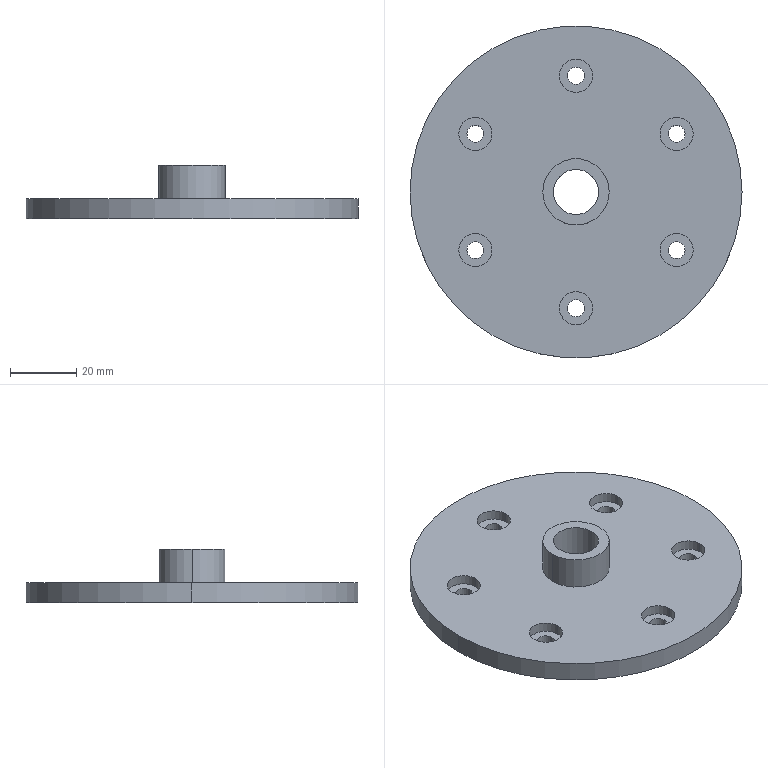Part | NX | 1 solid | 38 faces | box 100 x 100 x 16 mm | volume 46160 mm3 | cylinder 29 | plane 9 | commonest cylinder face diameters 5.1 x12 10 x12 20 x2 100 x2 13.6 x1
STEP:
#1=CARTESIAN_POINT('',(5.,-35.,3.));
#2=VERTEX_POINT('',#1);
#3=CARTESIAN_POINT('',(-5.,-35.,3.));
#4=VERTEX_POINT('',#3);
#5=CARTESIAN_POINT('',(0.,-35.,3.));
#6=DIRECTION('',(0.,0.,1.));
#7=DIRECTION('',(1.,0.,0.));
#8=AXIS2_PLACEMENT_3D('',#5,#6,#7);
#9=CIRCLE('',#8,5.);
#10=EDGE_CURVE('',#2,#4,#9,.T.);
#11=ORIENTED_EDGE('',*,*,#10,.T.);
#12=CARTESIAN_POINT('',(0.,-35.,3.));
#13=DIRECTION('',(0.,0.,1.));
#14=DIRECTION('',(1.,0.,0.));
#15=AXIS2_PLACEMENT_3D('',#12,#13,#14);
#16=CIRCLE('',#15,5.);
#17=EDGE_CURVE('',#4,#2,#16,.T.);
#18=ORIENTED_EDGE('',*,*,#17,.T.);
#19=EDGE_LOOP('',(#11,#18));
#20=FACE_BOUND('',#19,.T.);
#21=CARTESIAN_POINT('',(-2.55,-35.,3.));
#22=VERTEX_POINT('',#21);
#23=CARTESIAN_POINT('',(2.55,-35.,3.));
#24=VERTEX_POINT('',#23);
#25=CARTESIAN_POINT('',(0.,-35.,3.));
#26=DIRECTION('',(0.,0.,1.));
#27=DIRECTION('',(1.,0.,0.));
#28=AXIS2_PLACEMENT_3D('',#25,#26,#27);
#29=CIRCLE('',#28,2.55);
#30=EDGE_CURVE('',#22,#24,#29,.T.);
#31=ORIENTED_EDGE('',*,*,#30,.F.);
#32=CARTESIAN_POINT('',(0.,-35.,3.));
#33=DIRECTION('',(0.,0.,1.));
#34=DIRECTION('',(1.,0.,0.));
#35=AXIS2_PLACEMENT_3D('',#32,#33,#34);
#36=CIRCLE('',#35,2.55);
#37=EDGE_CURVE('',#24,#22,#36,.T.);
#38=ORIENTED_EDGE('',*,*,#37,.F.);
#39=EDGE_LOOP('',(#31,#38));
#40=FACE_BOUND('',#39,.T.);
#41=CARTESIAN_POINT('',(0.,-35.,3.));
#42=DIRECTION('',(0.,0.,1.));
#43=DIRECTION('',(1.,0.,0.));
#44=AXIS2_PLACEMENT_3D('',#41,#42,#43);
#45=PLANE('',#44);
#46=ADVANCED_FACE('',(#20,#40),#45,.T.);
#47=CARTESIAN_POINT('',(-5.,-35.,6.));
#48=VERTEX_POINT('',#47);
#49=CARTESIAN_POINT('',(-5.,-35.,3.));
#50=DIRECTION('',(0.,0.,1.));
#51=VECTOR('',#50,1000.);
#52=LINE('',#49,#51);
#53=EDGE_CURVE('',#4,#48,#52,.T.);
#54=ORIENTED_EDGE('',*,*,#53,.F.);
#55=ORIENTED_EDGE('',*,*,#10,.F.);
#56=CARTESIAN_POINT('',(5.,-35.,6.));
#57=VERTEX_POINT('',#56);
#58=CARTESIAN_POINT('',(5.,-35.,3.));
#59=DIRECTION('',(0.,0.,1.));
#60=VECTOR('',#59,1000.);
#61=LINE('',#58,#60);
#62=EDGE_CURVE('',#2,#57,#61,.T.);
#63=ORIENTED_EDGE('',*,*,#62,.T.);
#64=CARTESIAN_POINT('',(0.,-35.,6.));
#65=DIRECTION('',(0.,0.,1.));
#66=DIRECTION('',(1.,0.,0.));
#67=AXIS2_PLACEMENT_3D('',#64,#65,#66);
#68=CIRCLE('',#67,5.);
#69=EDGE_CURVE('',#57,#48,#68,.T.);
#70=ORIENTED_EDGE('',*,*,#69,.T.);
#71=EDGE_LOOP('',(#54,#55,#63,#70));
#72=FACE_BOUND('',#71,.T.);
#73=CARTESIAN_POINT('',(0.,-35.,3.));
#74=DIRECTION('',(0.,0.,1.));
#75=DIRECTION('',(1.,0.,0.));
#76=AXIS2_PLACEMENT_3D('',#73,#74,#75);
#77=CYLINDRICAL_SURFACE('',#76,5.);
#78=ADVANCED_FACE('',(#72),#77,.F.);
#79=CARTESIAN_POINT('',(5.,35.,3.));
#80=VERTEX_POINT('',#79);
#81=CARTESIAN_POINT('',(-5.,35.,3.));
#82=VERTEX_POINT('',#81);
#83=CARTESIAN_POINT('',(0.,35.,3.));
#84=DIRECTION('',(0.,0.,1.));
#85=DIRECTION('',(1.,0.,0.));
#86=AXIS2_PLACEMENT_3D('',#83,#84,#85);
#87=CIRCLE('',#86,5.);
#88=EDGE_CURVE('',#80,#82,#87,.T.);
#89=ORIENTED_EDGE('',*,*,#88,.T.);
#90=CARTESIAN_POINT('',(0.,35.,3.));
#91=DIRECTION('',(0.,0.,1.));
#92=DIRECTION('',(1.,0.,0.));
#93=AXIS2_PLACEMENT_3D('',#90,#91,#92);
#94=CIRCLE('',#93,5.);
#95=EDGE_CURVE('',#82,#80,#94,.T.);
#96=ORIENTED_EDGE('',*,*,#95,.T.);
#97=EDGE_LOOP('',(#89,#96));
#98=FACE_BOUND('',#97,.T.);
#99=CARTESIAN_POINT('',(-2.55,35.,3.));
#100=VERTEX_POINT('',#99);
#101=CARTESIAN_POINT('',(2.55,35.,3.));
#102=VERTEX_POINT('',#101);
#103=CARTESIAN_POINT('',(0.,35.,3.));
#104=DIRECTION('',(0.,0.,1.));
#105=DIRECTION('',(1.,0.,0.));
#106=AXIS2_PLACEMENT_3D('',#103,#104,#105);
#107=CIRCLE('',#106,2.55);
#108=EDGE_CURVE('',#100,#102,#107,.T.);
#109=ORIENTED_EDGE('',*,*,#108,.F.);
#110=CARTESIAN_POINT('',(0.,35.,3.));
#111=DIRECTION('',(0.,0.,1.));
#112=DIRECTION('',(1.,0.,0.));
#113=AXIS2_PLACEMENT_3D('',#110,#111,#112);
#114=CIRCLE('',#113,2.55);
#115=EDGE_CURVE('',#102,#100,#114,.T.);
#116=ORIENTED_EDGE('',*,*,#115,.F.);
#117=EDGE_LOOP('',(#109,#116));
#118=FACE_BOUND('',#117,.T.);
#119=CARTESIAN_POINT('',(0.,35.,3.));
#120=DIRECTION('',(0.,0.,1.));
#121=DIRECTION('',(1.,0.,0.));
#122=AXIS2_PLACEMENT_3D('',#119,#120,#121);
#123=PLANE('',#122);
#124=ADVANCED_FACE('',(#98,#118),#123,.T.);
#125=CARTESIAN_POINT('',(-5.,35.,6.));
#126=VERTEX_POINT('',#125);
#127=CARTESIAN_POINT('',(-5.,35.,3.));
#128=DIRECTION('',(0.,0.,1.));
#129=VECTOR('',#128,1000.);
#130=LINE('',#127,#129);
#131=EDGE_CURVE('',#82,#126,#130,.T.);
#132=ORIENTED_EDGE('',*,*,#131,.F.);
#133=ORIENTED_EDGE('',*,*,#88,.F.);
#134=CARTESIAN_POINT('',(5.,35.,6.));
#135=VERTEX_POINT('',#134);
#136=CARTESIAN_POINT('',(5.,35.,3.));
#137=DIRECTION('',(0.,0.,1.));
#138=VECTOR('',#137,1000.);
#139=LINE('',#136,#138);
#140=EDGE_CURVE('',#80,#135,#139,.T.);
#141=ORIENTED_EDGE('',*,*,#140,.T.);
#142=CARTESIAN_POINT('',(0.,35.,6.));
#143=DIRECTION('',(0.,0.,1.));
#144=DIRECTION('',(1.,0.,0.));
#145=AXIS2_PLACEMENT_3D('',#142,#143,#144);
#146=CIRCLE('',#145,5.);
#147=EDGE_CURVE('',#135,#126,#146,.T.);
#148=ORIENTED_EDGE('',*,*,#147,.T.);
#149=EDGE_LOOP('',(#132,#133,#141,#148));
#150=FACE_BOUND('',#149,.T.);
#151=CARTESIAN_POINT('',(0.,35.,3.));
#152=DIRECTION('',(0.,0.,1.));
#153=DIRECTION('',(1.,0.,0.));
#154=AXIS2_PLACEMENT_3D('',#151,#152,#153);
#155=CYLINDRICAL_SURFACE('',#154,5.);
#156=ADVANCED_FACE('',(#150),#155,.F.);
#157=CARTESIAN_POINT('',(35.311,17.5,3.));
#158=VERTEX_POINT('',#157);
#159=CARTESIAN_POINT('',(25.311,17.5,3.));
#160=VERTEX_POINT('',#159);
#161=CARTESIAN_POINT('',(30.311,17.5,3.));
#162=DIRECTION('',(0.,0.,1.));
#163=DIRECTION('',(1.,0.,0.));
#164=AXIS2_PLACEMENT_3D('',#161,#162,#163);
#165=CIRCLE('',#164,5.);
#166=EDGE_CURVE('',#158,#160,#165,.T.);
#167=ORIENTED_EDGE('',*,*,#166,.T.);
#168=CARTESIAN_POINT('',(30.311,17.5,3.));
#169=DIRECTION('',(0.,0.,1.));
#170=DIRECTION('',(1.,0.,0.));
#171=AXIS2_PLACEMENT_3D('',#168,#169,#170);
#172=CIRCLE('',#171,5.);
#173=EDGE_CURVE('',#160,#158,#172,.T.);
#174=ORIENTED_EDGE('',*,*,#173,.T.);
#175=EDGE_LOOP('',(#167,#174));
#176=FACE_BOUND('',#175,.T.);
#177=CARTESIAN_POINT('',(27.761,17.5,3.));
#178=VERTEX_POINT('',#177);
#179=CARTESIAN_POINT('',(32.861,17.5,3.));
#180=VERTEX_POINT('',#179);
#181=CARTESIAN_POINT('',(30.311,17.5,3.));
#182=DIRECTION('',(0.,0.,1.));
#183=DIRECTION('',(1.,0.,0.));
#184=AXIS2_PLACEMENT_3D('',#181,#182,#183);
#185=CIRCLE('',#184,2.55);
#186=EDGE_CURVE('',#178,#180,#185,.T.);
#187=ORIENTED_EDGE('',*,*,#186,.F.);
#188=CARTESIAN_POINT('',(30.311,17.5,3.));
#189=DIRECTION('',(0.,0.,1.));
#190=DIRECTION('',(1.,0.,0.));
#191=AXIS2_PLACEMENT_3D('',#188,#189,#190);
#192=CIRCLE('',#191,2.55);
#193=EDGE_CURVE('',#180,#178,#192,.T.);
#194=ORIENTED_EDGE('',*,*,#193,.F.);
#195=EDGE_LOOP('',(#187,#194));
#196=FACE_BOUND('',#195,.T.);
#197=CARTESIAN_POINT('',(30.311,17.5,3.));
#198=DIRECTION('',(0.,0.,1.));
#199=DIRECTION('',(1.,0.,0.));
#200=AXIS2_PLACEMENT_3D('',#197,#198,#199);
#201=PLANE('',#200);
#202=ADVANCED_FACE('',(#176,#196),#201,.T.);
#203=CARTESIAN_POINT('',(25.311,17.5,6.));
#204=VERTEX_POINT('',#203);
#205=CARTESIAN_POINT('',(25.311,17.5,3.));
#206=DIRECTION('',(0.,0.,1.));
#207=VECTOR('',#206,1000.);
#208=LINE('',#205,#207);
#209=EDGE_CURVE('',#160,#204,#208,.T.);
#210=ORIENTED_EDGE('',*,*,#209,.F.);
#211=ORIENTED_EDGE('',*,*,#166,.F.);
#212=CARTESIAN_POINT('',(35.311,17.5,6.));
#213=VERTEX_POINT('',#212);
#214=CARTESIAN_POINT('',(35.311,17.5,3.));
#215=DIRECTION('',(0.,0.,1.));
#216=VECTOR('',#215,1000.);
#217=LINE('',#214,#216);
#218=EDGE_CURVE('',#158,#213,#217,.T.);
#219=ORIENTED_EDGE('',*,*,#218,.T.);
#220=CARTESIAN_POINT('',(30.311,17.5,6.));
#221=DIRECTION('',(0.,0.,1.));
#222=DIRECTION('',(1.,0.,0.));
#223=AXIS2_PLACEMENT_3D('',#220,#221,#222);
#224=CIRCLE('',#223,5.);
#225=EDGE_CURVE('',#213,#204,#224,.T.);
#226=ORIENTED_EDGE('',*,*,#225,.T.);
#227=EDGE_LOOP('',(#210,#211,#219,#226));
#228=FACE_BOUND('',#227,.T.);
#229=CARTESIAN_POINT('',(30.311,17.5,3.));
#230=DIRECTION('',(0.,0.,1.));
#231=DIRECTION('',(1.,0.,0.));
#232=AXIS2_PLACEMENT_3D('',#229,#230,#231);
#233=CYLINDRICAL_SURFACE('',#232,5.);
#234=ADVANCED_FACE('',(#228),#233,.F.);
#235=CARTESIAN_POINT('',(35.311,-17.5,3.));
#236=VERTEX_POINT('',#235);
#237=CARTESIAN_POINT('',(25.311,-17.5,3.));
#238=VERTEX_POINT('',#237);
#239=CARTESIAN_POINT('',(30.311,-17.5,3.));
#240=DIRECTION('',(0.,0.,1.));
#241=DIRECTION('',(1.,0.,0.));
#242=AXIS2_PLACEMENT_3D('',#239,#240,#241);
#243=CIRCLE('',#242,5.);
#244=EDGE_CURVE('',#236,#238,#243,.T.);
#245=ORIENTED_EDGE('',*,*,#244,.T.);
#246=CARTESIAN_POINT('',(30.311,-17.5,3.));
#247=DIRECTION('',(0.,0.,1.));
#248=DIRECTION('',(1.,0.,0.));
#249=AXIS2_PLACEMENT_3D('',#246,#247,#248);
#250=CIRCLE('',#249,5.);
#251=EDGE_CURVE('',#238,#236,#250,.T.);
#252=ORIENTED_EDGE('',*,*,#251,.T.);
#253=EDGE_LOOP('',(#245,#252));
#254=FACE_BOUND('',#253,.T.);
#255=CARTESIAN_POINT('',(27.761,-17.5,3.));
#256=VERTEX_POINT('',#255);
#257=CARTESIAN_POINT('',(32.861,-17.5,3.));
#258=VERTEX_POINT('',#257);
#259=CARTESIAN_POINT('',(30.311,-17.5,3.));
#260=DIRECTION('',(0.,0.,1.));
#261=DIRECTION('',(1.,0.,0.));
#262=AXIS2_PLACEMENT_3D('',#259,#260,#261);
#263=CIRCLE('',#262,2.55);
#264=EDGE_CURVE('',#256,#258,#263,.T.);
#265=ORIENTED_EDGE('',*,*,#264,.F.);
#266=CARTESIAN_POINT('',(30.311,-17.5,3.));
#267=DIRECTION('',(0.,0.,1.));
#268=DIRECTION('',(1.,0.,0.));
#269=AXIS2_PLACEMENT_3D('',#266,#267,#268);
#270=CIRCLE('',#269,2.55);
#271=EDGE_CURVE('',#258,#256,#270,.T.);
#272=ORIENTED_EDGE('',*,*,#271,.F.);
#273=EDGE_LOOP('',(#265,#272));
#274=FACE_BOUND('',#273,.T.);
#275=CARTESIAN_POINT('',(30.311,-17.5,3.));
#276=DIRECTION('',(0.,0.,1.));
#277=DIRECTION('',(1.,0.,0.));
#278=AXIS2_PLACEMENT_3D('',#275,#276,#277);
#279=PLANE('',#278);
#280=ADVANCED_FACE('',(#254,#274),#279,.T.);
#281=CARTESIAN_POINT('',(25.311,-17.5,6.));
#282=VERTEX_POINT('',#281);
#283=CARTESIAN_POINT('',(25.311,-17.5,3.));
#284=DIRECTION('',(0.,0.,1.));
#285=VECTOR('',#284,1000.);
#286=LINE('',#283,#285);
#287=EDGE_CURVE('',#238,#282,#286,.T.);
#288=ORIENTED_EDGE('',*,*,#287,.F.);
#289=ORIENTED_EDGE('',*,*,#244,.F.);
#290=CARTESIAN_POINT('',(35.311,-17.5,6.));
#291=VERTEX_POINT('',#290);
#292=CARTESIAN_POINT('',(35.311,-17.5,3.));
#293=DIRECTION('',(0.,0.,1.));
#294=VECTOR('',#293,1000.);
#295=LINE('',#292,#294);
#296=EDGE_CURVE('',#236,#291,#295,.T.);
#297=ORIENTED_EDGE('',*,*,#296,.T.);
#298=CARTESIAN_POINT('',(30.311,-17.5,6.));
#299=DIRECTION('',(0.,0.,1.));
#300=DIRECTION('',(1.,0.,0.));
#301=AXIS2_PLACEMENT_3D('',#298,#299,#300);
#302=CIRCLE('',#301,5.);
#303=EDGE_CURVE('',#291,#282,#302,.T.);
#304=ORIENTED_EDGE('',*,*,#303,.T.);
#305=EDGE_LOOP('',(#288,#289,#297,#304));
#306=FACE_BOUND('',#305,.T.);
#307=CARTESIAN_POINT('',(30.311,-17.5,3.));
#308=DIRECTION('',(0.,0.,1.));
#309=DIRECTION('',(1.,0.,0.));
#310=AXIS2_PLACEMENT_3D('',#307,#308,#309);
#311=CYLINDRICAL_SURFACE('',#310,5.);
#312=ADVANCED_FACE('',(#306),#311,.F.);
#313=CARTESIAN_POINT('',(-25.311,-17.5,3.));
#314=VERTEX_POINT('',#313);
#315=CARTESIAN_POINT('',(-35.311,-17.5,3.));
#316=VERTEX_POINT('',#315);
#317=CARTESIAN_POINT('',(-30.311,-17.5,3.));
#318=DIRECTION('',(0.,0.,1.));
#319=DIRECTION('',(1.,0.,0.));
#320=AXIS2_PLACEMENT_3D('',#317,#318,#319);
#321=CIRCLE('',#320,5.);
#322=EDGE_CURVE('',#314,#316,#321,.T.);
#323=ORIENTED_EDGE('',*,*,#322,.T.);
#324=CARTESIAN_POINT('',(-30.311,-17.5,3.));
#325=DIRECTION('',(0.,0.,1.));
#326=DIRECTION('',(1.,0.,0.));
#327=AXIS2_PLACEMENT_3D('',#324,#325,#326);
#328=CIRCLE('',#327,5.);
#329=EDGE_CURVE('',#316,#314,#328,.T.);
#330=ORIENTED_EDGE('',*,*,#329,.T.);
#331=EDGE_LOOP('',(#323,#330));
#332=FACE_BOUND('',#331,.T.);
#333=CARTESIAN_POINT('',(-32.861,-17.5,3.));
#334=VERTEX_POINT('',#333);
#335=CARTESIAN_POINT('',(-27.761,-17.5,3.));
#336=VERTEX_POINT('',#335);
#337=CARTESIAN_POINT('',(-30.311,-17.5,3.));
#338=DIRECTION('',(0.,0.,1.));
#339=DIRECTION('',(1.,0.,0.));
#340=AXIS2_PLACEMENT_3D('',#337,#338,#339);
#341=CIRCLE('',#340,2.55);
#342=EDGE_CURVE('',#334,#336,#341,.T.);
#343=ORIENTED_EDGE('',*,*,#342,.F.);
#344=CARTESIAN_POINT('',(-30.311,-17.5,3.));
#345=DIRECTION('',(0.,0.,1.));
#346=DIRECTION('',(1.,0.,0.));
#347=AXIS2_PLACEMENT_3D('',#344,#345,#346);
#348=CIRCLE('',#347,2.55);
#349=EDGE_CURVE('',#336,#334,#348,.T.);
#350=ORIENTED_EDGE('',*,*,#349,.F.);
#351=EDGE_LOOP('',(#343,#350));
#352=FACE_BOUND('',#351,.T.);
#353=CARTESIAN_POINT('',(-30.311,-17.5,3.));
#354=DIRECTION('',(0.,0.,1.));
#355=DIRECTION('',(1.,0.,0.));
#356=AXIS2_PLACEMENT_3D('',#353,#354,#355);
#357=PLANE('',#356);
#358=ADVANCED_FACE('',(#332,#352),#357,.T.);
#359=CARTESIAN_POINT('',(-35.311,-17.5,6.));
#360=VERTEX_POINT('',#359);
#361=CARTESIAN_POINT('',(-35.311,-17.5,3.));
#362=DIRECTION('',(0.,0.,1.));
#363=VECTOR('',#362,1000.);
#364=LINE('',#361,#363);
#365=EDGE_CURVE('',#316,#360,#364,.T.);
#366=ORIENTED_EDGE('',*,*,#365,.F.);
#367=ORIENTED_EDGE('',*,*,#322,.F.);
#368=CARTESIAN_POINT('',(-25.311,-17.5,6.));
#369=VERTEX_POINT('',#368);
#370=CARTESIAN_POINT('',(-25.311,-17.5,3.));
#371=DIRECTION('',(0.,0.,1.));
#372=VECTOR('',#371,1000.);
#373=LINE('',#370,#372);
#374=EDGE_CURVE('',#314,#369,#373,.T.);
#375=ORIENTED_EDGE('',*,*,#374,.T.);
#376=CARTESIAN_POINT('',(-30.311,-17.5,6.));
#377=DIRECTION('',(0.,0.,1.));
#378=DIRECTION('',(1.,0.,0.));
#379=AXIS2_PLACEMENT_3D('',#376,#377,#378);
#380=CIRCLE('',#379,5.);
#381=EDGE_CURVE('',#369,#360,#380,.T.);
#382=ORIENTED_EDGE('',*,*,#381,.T.);
#383=EDGE_LOOP('',(#366,#367,#375,#382));
#384=FACE_BOUND('',#383,.T.);
#385=CARTESIAN_POINT('',(-30.311,-17.5,3.));
#386=DIRECTION('',(0.,0.,1.));
#387=DIRECTION('',(1.,0.,0.));
#388=AXIS2_PLACEMENT_3D('',#385,#386,#387);
#389=CYLINDRICAL_SURFACE('',#388,5.);
#390=ADVANCED_FACE('',(#384),#389,.F.);
#391=CARTESIAN_POINT('',(-25.311,17.5,3.));
#392=VERTEX_POINT('',#391);
#393=CARTESIAN_POINT('',(-35.311,17.5,3.));
#394=VERTEX_POINT('',#393);
#395=CARTESIAN_POINT('',(-30.311,17.5,3.));
#396=DIRECTION('',(0.,0.,1.));
#397=DIRECTION('',(1.,0.,0.));
#398=AXIS2_PLACEMENT_3D('',#395,#396,#397);
#399=CIRCLE('',#398,5.);
#400=EDGE_CURVE('',#392,#394,#399,.T.);
#401=ORIENTED_EDGE('',*,*,#400,.T.);
#402=CARTESIAN_POINT('',(-30.311,17.5,3.));
#403=DIRECTION('',(0.,0.,1.));
#404=DIRECTION('',(1.,0.,0.));
#405=AXIS2_PLACEMENT_3D('',#402,#403,#404);
#406=CIRCLE('',#405,5.);
#407=EDGE_CURVE('',#394,#392,#406,.T.);
#408=ORIENTED_EDGE('',*,*,#407,.T.);
#409=EDGE_LOOP('',(#401,#408));
#410=FACE_BOUND('',#409,.T.);
#411=CARTESIAN_POINT('',(-32.861,17.5,3.));
#412=VERTEX_POINT('',#411);
#413=CARTESIAN_POINT('',(-27.761,17.5,3.));
#414=VERTEX_POINT('',#413);
#415=CARTESIAN_POINT('',(-30.311,17.5,3.));
#416=DIRECTION('',(0.,0.,1.));
#417=DIRECTION('',(1.,0.,0.));
#418=AXIS2_PLACEMENT_3D('',#415,#416,#417);
#419=CIRCLE('',#418,2.55);
#420=EDGE_CURVE('',#412,#414,#419,.T.);
#421=ORIENTED_EDGE('',*,*,#420,.F.);
#422=CARTESIAN_POINT('',(-30.311,17.5,3.));
#423=DIRECTION('',(0.,0.,1.));
#424=DIRECTION('',(1.,0.,0.));
#425=AXIS2_PLACEMENT_3D('',#422,#423,#424);
#426=CIRCLE('',#425,2.55);
#427=EDGE_CURVE('',#414,#412,#426,.T.);
#428=ORIENTED_EDGE('',*,*,#427,.F.);
#429=EDGE_LOOP('',(#421,#428));
#430=FACE_BOUND('',#429,.T.);
#431=CARTESIAN_POINT('',(-30.311,17.5,3.));
#432=DIRECTION('',(0.,0.,1.));
#433=DIRECTION('',(1.,0.,0.));
#434=AXIS2_PLACEMENT_3D('',#431,#432,#433);
#435=PLANE('',#434);
#436=ADVANCED_FACE('',(#410,#430),#435,.T.);
#437=CARTESIAN_POINT('',(-35.311,17.5,6.));
#438=VERTEX_POINT('',#437);
#439=CARTESIAN_POINT('',(-35.311,17.5,3.));
#440=DIRECTION('',(0.,0.,1.));
#441=VECTOR('',#440,1000.);
#442=LINE('',#439,#441);
#443=EDGE_CURVE('',#394,#438,#442,.T.);
#444=ORIENTED_EDGE('',*,*,#443,.F.);
#445=ORIENTED_EDGE('',*,*,#400,.F.);
#446=CARTESIAN_POINT('',(-25.311,17.5,6.));
#447=VERTEX_POINT('',#446);
#448=CARTESIAN_POINT('',(-25.311,17.5,3.));
#449=DIRECTION('',(0.,0.,1.));
#450=VECTOR('',#449,1000.);
#451=LINE('',#448,#450);
#452=EDGE_CURVE('',#392,#447,#451,.T.);
#453=ORIENTED_EDGE('',*,*,#452,.T.);
#454=CARTESIAN_POINT('',(-30.311,17.5,6.));
#455=DIRECTION('',(0.,0.,1.));
#456=DIRECTION('',(1.,0.,0.));
#457=AXIS2_PLACEMENT_3D('',#454,#455,#456);
#458=CIRCLE('',#457,5.);
#459=EDGE_CURVE('',#447,#438,#458,.T.);
#460=ORIENTED_EDGE('',*,*,#459,.T.);
#461=EDGE_LOOP('',(#444,#445,#453,#460));
#462=FACE_BOUND('',#461,.T.);
#463=CARTESIAN_POINT('',(-30.311,17.5,3.));
#464=DIRECTION('',(0.,0.,1.));
#465=DIRECTION('',(1.,0.,0.));
#466=AXIS2_PLACEMENT_3D('',#463,#464,#465);
#467=CYLINDRICAL_SURFACE('',#466,5.);
#468=ADVANCED_FACE('',(#462),#467,.F.);
#469=CARTESIAN_POINT('',(10.,0.,16.));
#470=VERTEX_POINT('',#469);
#471=CARTESIAN_POINT('',(10.,0.,6.));
#472=VERTEX_POINT('',#471);
#473=CARTESIAN_POINT('',(10.,0.,16.));
#474=DIRECTION('',(0.,0.,-1.));
#475=VECTOR('',#474,1000.);
#476=LINE('',#473,#475);
#477=EDGE_CURVE('',#470,#472,#476,.T.);
#478=ORIENTED_EDGE('',*,*,#477,.F.);
#479=CARTESIAN_POINT('',(-10.,0.,16.));
#480=VERTEX_POINT('',#479);
#481=CARTESIAN_POINT('',(0.,0.,16.));
#482=DIRECTION('',(0.,0.,1.));
#483=DIRECTION('',(1.,0.,0.));
#484=AXIS2_PLACEMENT_3D('',#481,#482,#483);
#485=CIRCLE('',#484,10.);
#486=EDGE_CURVE('',#480,#470,#485,.T.);
#487=ORIENTED_EDGE('',*,*,#486,.F.);
#488=CARTESIAN_POINT('',(-10.,0.,6.));
#489=VERTEX_POINT('',#488);
#490=CARTESIAN_POINT('',(-10.,0.,16.));
#491=DIRECTION('',(0.,0.,-1.));
#492=VECTOR('',#491,1000.);
#493=LINE('',#490,#492);
#494=EDGE_CURVE('',#480,#489,#493,.T.);
#495=ORIENTED_EDGE('',*,*,#494,.T.);
#496=CARTESIAN_POINT('',(0.,0.,6.));
#497=DIRECTION('',(0.,0.,1.));
#498=DIRECTION('',(1.,0.,0.));
#499=AXIS2_PLACEMENT_3D('',#496,#497,#498);
#500=CIRCLE('',#499,10.);
#501=EDGE_CURVE('',#489,#472,#500,.T.);
#502=ORIENTED_EDGE('',*,*,#501,.T.);
#503=EDGE_LOOP('',(#478,#487,#495,#502));
#504=FACE_BOUND('',#503,.T.);
#505=CARTESIAN_POINT('',(0.,0.,16.));
#506=DIRECTION('',(0.,0.,-1.));
#507=DIRECTION('',(-1.,0.,0.));
#508=AXIS2_PLACEMENT_3D('',#505,#506,#507);
#509=CYLINDRICAL_SURFACE('',#508,10.);
#510=ADVANCED_FACE('',(#504),#509,.T.);
#511=CARTESIAN_POINT('',(6.8,0.,16.));
#512=VERTEX_POINT('',#511);
#513=CARTESIAN_POINT('',(0.,0.,16.));
#514=DIRECTION('',(0.,0.,1.));
#515=DIRECTION('',(1.,0.,0.));
#516=AXIS2_PLACEMENT_3D('',#513,#514,#515);
#517=CIRCLE('',#516,6.8);
#518=EDGE_CURVE('',#512,#512,#517,.T.);
#519=ORIENTED_EDGE('',*,*,#518,.F.);
#520=EDGE_LOOP('',(#519));
#521=FACE_BOUND('',#520,.T.);
#522=ORIENTED_EDGE('',*,*,#486,.T.);
#523=CARTESIAN_POINT('',(0.,0.,16.));
#524=DIRECTION('',(0.,0.,1.));
#525=DIRECTION('',(1.,0.,0.));
#526=AXIS2_PLACEMENT_3D('',#523,#524,#525);
#527=CIRCLE('',#526,10.);
#528=EDGE_CURVE('',#470,#480,#527,.T.);
#529=ORIENTED_EDGE('',*,*,#528,.T.);
#530=EDGE_LOOP('',(#522,#529));
#531=FACE_BOUND('',#530,.T.);
#532=CARTESIAN_POINT('',(0.,0.,16.));
#533=DIRECTION('',(0.,0.,1.));
#534=DIRECTION('',(1.,0.,0.));
#535=AXIS2_PLACEMENT_3D('',#532,#533,#534);
#536=PLANE('',#535);
#537=ADVANCED_FACE('',(#521,#531),#536,.T.);
#538=CARTESIAN_POINT('',(50.,0.,6.));
#539=VERTEX_POINT('',#538);
#540=CARTESIAN_POINT('',(50.,0.,0.));
#541=VERTEX_POINT('',#540);
#542=CARTESIAN_POINT('',(50.,0.,6.));
#543=DIRECTION('',(0.,0.,-1.));
#544=VECTOR('',#543,1000.);
#545=LINE('',#542,#544);
#546=EDGE_CURVE('',#539,#541,#545,.T.);
#547=ORIENTED_EDGE('',*,*,#546,.F.);
#548=CARTESIAN_POINT('',(-50.,0.,6.));
#549=VERTEX_POINT('',#548);
#550=CARTESIAN_POINT('',(0.,0.,6.));
#551=DIRECTION('',(0.,0.,1.));
#552=DIRECTION('',(1.,0.,0.));
#553=AXIS2_PLACEMENT_3D('',#550,#551,#552);
#554=CIRCLE('',#553,50.);
#555=EDGE_CURVE('',#549,#539,#554,.T.);
#556=ORIENTED_EDGE('',*,*,#555,.F.);
#557=CARTESIAN_POINT('',(-50.,0.,0.));
#558=VERTEX_POINT('',#557);
#559=CARTESIAN_POINT('',(-50.,0.,6.));
#560=DIRECTION('',(0.,0.,-1.));
#561=VECTOR('',#560,1000.);
#562=LINE('',#559,#561);
#563=EDGE_CURVE('',#549,#558,#562,.T.);
#564=ORIENTED_EDGE('',*,*,#563,.T.);
#565=CARTESIAN_POINT('',(0.,0.,0.));
#566=DIRECTION('',(0.,0.,1.));
#567=DIRECTION('',(1.,0.,0.));
#568=AXIS2_PLACEMENT_3D('',#565,#566,#567);
#569=CIRCLE('',#568,50.);
#570=EDGE_CURVE('',#558,#541,#569,.T.);
#571=ORIENTED_EDGE('',*,*,#570,.T.);
#572=EDGE_LOOP('',(#547,#556,#564,#571));
#573=FACE_BOUND('',#572,.T.);
#574=CARTESIAN_POINT('',(0.,0.,6.));
#575=DIRECTION('',(0.,0.,-1.));
#576=DIRECTION('',(-1.,0.,0.));
#577=AXIS2_PLACEMENT_3D('',#574,#575,#576);
#578=CYLINDRICAL_SURFACE('',#577,50.);
#579=ADVANCED_FACE('',(#573),#578,.T.);
#580=CARTESIAN_POINT('',(-32.861,17.5,0.));
#581=VERTEX_POINT('',#580);
#582=CARTESIAN_POINT('',(-27.761,17.5,0.));
#583=VERTEX_POINT('',#582);
#584=CARTESIAN_POINT('',(-30.311,17.5,0.));
#585=DIRECTION('',(0.,0.,1.));
#586=DIRECTION('',(1.,0.,0.));
#587=AXIS2_PLACEMENT_3D('',#584,#585,#586);
#588=CIRCLE('',#587,2.55);
#589=EDGE_CURVE('',#581,#583,#588,.T.);
#590=ORIENTED_EDGE('',*,*,#589,.T.);
#591=CARTESIAN_POINT('',(-30.311,17.5,0.));
#592=DIRECTION('',(0.,0.,1.));
#593=DIRECTION('',(1.,0.,0.));
#594=AXIS2_PLACEMENT_3D('',#591,#592,#593);
#595=CIRCLE('',#594,2.55);
#596=EDGE_CURVE('',#583,#581,#595,.T.);
#597=ORIENTED_EDGE('',*,*,#596,.T.);
#598=EDGE_LOOP('',(#590,#597));
#599=FACE_BOUND('',#598,.T.);
#600=CARTESIAN_POINT('',(-32.861,-17.5,0.));
#601=VERTEX_POINT('',#600);
#602=CARTESIAN_POINT('',(-27.761,-17.5,0.));
#603=VERTEX_POINT('',#602);
#604=CARTESIAN_POINT('',(-30.311,-17.5,0.));
#605=DIRECTION('',(0.,0.,1.));
#606=DIRECTION('',(1.,0.,0.));
#607=AXIS2_PLACEMENT_3D('',#604,#605,#606);
#608=CIRCLE('',#607,2.55);
#609=EDGE_CURVE('',#601,#603,#608,.T.);
#610=ORIENTED_EDGE('',*,*,#609,.T.);
#611=CARTESIAN_POINT('',(-30.311,-17.5,0.));
#612=DIRECTION('',(0.,0.,1.));
#613=DIRECTION('',(1.,0.,0.));
#614=AXIS2_PLACEMENT_3D('',#611,#612,#613);
#615=CIRCLE('',#614,2.55);
#616=EDGE_CURVE('',#603,#601,#615,.T.);
#617=ORIENTED_EDGE('',*,*,#616,.T.);
#618=EDGE_LOOP('',(#610,#617));
#619=FACE_BOUND('',#618,.T.);
#620=CARTESIAN_POINT('',(27.761,-17.5,0.));
#621=VERTEX_POINT('',#620);
#622=CARTESIAN_POINT('',(32.861,-17.5,0.));
#623=VERTEX_POINT('',#622);
#624=CARTESIAN_POINT('',(30.311,-17.5,0.));
#625=DIRECTION('',(0.,0.,1.));
#626=DIRECTION('',(1.,0.,0.));
#627=AXIS2_PLACEMENT_3D('',#624,#625,#626);
#628=CIRCLE('',#627,2.55);
#629=EDGE_CURVE('',#621,#623,#628,.T.);
#630=ORIENTED_EDGE('',*,*,#629,.T.);
#631=CARTESIAN_POINT('',(30.311,-17.5,0.));
#632=DIRECTION('',(0.,0.,1.));
#633=DIRECTION('',(1.,0.,0.));
#634=AXIS2_PLACEMENT_3D('',#631,#632,#633);
#635=CIRCLE('',#634,2.55);
#636=EDGE_CURVE('',#623,#621,#635,.T.);
#637=ORIENTED_EDGE('',*,*,#636,.T.);
#638=EDGE_LOOP('',(#630,#637));
#639=FACE_BOUND('',#638,.T.);
#640=CARTESIAN_POINT('',(27.761,17.5,0.));
#641=VERTEX_POINT('',#640);
#642=CARTESIAN_POINT('',(32.861,17.5,0.));
#643=VERTEX_POINT('',#642);
#644=CARTESIAN_POINT('',(30.311,17.5,0.));
#645=DIRECTION('',(0.,0.,1.));
#646=DIRECTION('',(1.,0.,0.));
#647=AXIS2_PLACEMENT_3D('',#644,#645,#646);
#648=CIRCLE('',#647,2.55);
#649=EDGE_CURVE('',#641,#643,#648,.T.);
#650=ORIENTED_EDGE('',*,*,#649,.T.);
#651=CARTESIAN_POINT('',(30.311,17.5,0.));
#652=DIRECTION('',(0.,0.,1.));
#653=DIRECTION('',(1.,0.,0.));
#654=AXIS2_PLACEMENT_3D('',#651,#652,#653);
#655=CIRCLE('',#654,2.55);
#656=EDGE_CURVE('',#643,#641,#655,.T.);
#657=ORIENTED_EDGE('',*,*,#656,.T.);
#658=EDGE_LOOP('',(#650,#657));
#659=FACE_BOUND('',#658,.T.);
#660=CARTESIAN_POINT('',(-2.55,35.,0.));
#661=VERTEX_POINT('',#660);
#662=CARTESIAN_POINT('',(2.55,35.,0.));
#663=VERTEX_POINT('',#662);
#664=CARTESIAN_POINT('',(0.,35.,0.));
#665=DIRECTION('',(0.,0.,1.));
#666=DIRECTION('',(1.,0.,0.));
#667=AXIS2_PLACEMENT_3D('',#664,#665,#666);
#668=CIRCLE('',#667,2.55);
#669=EDGE_CURVE('',#661,#663,#668,.T.);
#670=ORIENTED_EDGE('',*,*,#669,.T.);
#671=CARTESIAN_POINT('',(0.,35.,0.));
#672=DIRECTION('',(0.,0.,1.));
#673=DIRECTION('',(1.,0.,0.));
#674=AXIS2_PLACEMENT_3D('',#671,#672,#673);
#675=CIRCLE('',#674,2.55);
#676=EDGE_CURVE('',#663,#661,#675,.T.);
#677=ORIENTED_EDGE('',*,*,#676,.T.);
#678=EDGE_LOOP('',(#670,#677));
#679=FACE_BOUND('',#678,.T.);
#680=CARTESIAN_POINT('',(-2.55,-35.,0.));
#681=VERTEX_POINT('',#680);
#682=CARTESIAN_POINT('',(2.55,-35.,0.));
#683=VERTEX_POINT('',#682);
#684=CARTESIAN_POINT('',(0.,-35.,0.));
#685=DIRECTION('',(0.,0.,1.));
#686=DIRECTION('',(1.,0.,0.));
#687=AXIS2_PLACEMENT_3D('',#684,#685,#686);
#688=CIRCLE('',#687,2.55);
#689=EDGE_CURVE('',#681,#683,#688,.T.);
#690=ORIENTED_EDGE('',*,*,#689,.T.);
#691=CARTESIAN_POINT('',(0.,-35.,0.));
#692=DIRECTION('',(0.,0.,1.));
#693=DIRECTION('',(1.,0.,0.));
#694=AXIS2_PLACEMENT_3D('',#691,#692,#693);
#695=CIRCLE('',#694,2.55);
#696=EDGE_CURVE('',#683,#681,#695,.T.);
#697=ORIENTED_EDGE('',*,*,#696,.T.);
#698=EDGE_LOOP('',(#690,#697));
#699=FACE_BOUND('',#698,.T.);
#700=ORIENTED_EDGE('',*,*,#570,.F.);
#701=CARTESIAN_POINT('',(0.,0.,0.));
#702=DIRECTION('',(0.,0.,1.));
#703=DIRECTION('',(1.,0.,0.));
#704=AXIS2_PLACEMENT_3D('',#701,#702,#703);
#705=CIRCLE('',#704,50.);
#706=EDGE_CURVE('',#541,#558,#705,.T.);
#707=ORIENTED_EDGE('',*,*,#706,.F.);
#708=EDGE_LOOP('',(#700,#707));
#709=FACE_BOUND('',#708,.T.);
#710=CARTESIAN_POINT('',(6.8,0.,0.));
#711=VERTEX_POINT('',#710);
#712=CARTESIAN_POINT('',(0.,0.,0.));
#713=DIRECTION('',(0.,0.,1.));
#714=DIRECTION('',(1.,0.,0.));
#715=AXIS2_PLACEMENT_3D('',#712,#713,#714);
#716=CIRCLE('',#715,6.8);
#717=EDGE_CURVE('',#711,#711,#716,.T.);
#718=ORIENTED_EDGE('',*,*,#717,.T.);
#719=EDGE_LOOP('',(#718));
#720=FACE_BOUND('',#719,.T.);
#721=CARTESIAN_POINT('',(0.,0.,0.));
#722=DIRECTION('',(0.,0.,1.));
#723=DIRECTION('',(1.,0.,0.));
#724=AXIS2_PLACEMENT_3D('',#721,#722,#723);
#725=PLANE('',#724);
#726=ADVANCED_FACE('',(#599,#619,#639,#659,#679,#699,#709,#720),#725,.F.);
#727=ORIENTED_EDGE('',*,*,#555,.T.);
#728=CARTESIAN_POINT('',(0.,0.,6.));
#729=DIRECTION('',(0.,0.,1.));
#730=DIRECTION('',(1.,0.,0.));
#731=AXIS2_PLACEMENT_3D('',#728,#729,#730);
#732=CIRCLE('',#731,50.);
#733=EDGE_CURVE('',#539,#549,#732,.T.);
#734=ORIENTED_EDGE('',*,*,#733,.T.);
#735=EDGE_LOOP('',(#727,#734));
#736=FACE_BOUND('',#735,.T.);
#737=ORIENTED_EDGE('',*,*,#501,.F.);
#738=CARTESIAN_POINT('',(0.,0.,6.));
#739=DIRECTION('',(0.,0.,1.));
#740=DIRECTION('',(1.,0.,0.));
#741=AXIS2_PLACEMENT_3D('',#738,#739,#740);
#742=CIRCLE('',#741,10.);
#743=EDGE_CURVE('',#472,#489,#742,.T.);
#744=ORIENTED_EDGE('',*,*,#743,.F.);
#745=EDGE_LOOP('',(#737,#744));
#746=FACE_BOUND('',#745,.T.);
#747=ORIENTED_EDGE('',*,*,#381,.F.);
#748=CARTESIAN_POINT('',(-30.311,-17.5,6.));
#749=DIRECTION('',(0.,0.,1.));
#750=DIRECTION('',(1.,0.,0.));
#751=AXIS2_PLACEMENT_3D('',#748,#749,#750);
#752=CIRCLE('',#751,5.);
#753=EDGE_CURVE('',#360,#369,#752,.T.);
#754=ORIENTED_EDGE('',*,*,#753,.F.);
#755=EDGE_LOOP('',(#747,#754));
#756=FACE_BOUND('',#755,.T.);
#757=ORIENTED_EDGE('',*,*,#303,.F.);
#758=CARTESIAN_POINT('',(30.311,-17.5,6.));
#759=DIRECTION('',(0.,0.,1.));
#760=DIRECTION('',(1.,0.,0.));
#761=AXIS2_PLACEMENT_3D('',#758,#759,#760);
#762=CIRCLE('',#761,5.);
#763=EDGE_CURVE('',#282,#291,#762,.T.);
#764=ORIENTED_EDGE('',*,*,#763,.F.);
#765=EDGE_LOOP('',(#757,#764));
#766=FACE_BOUND('',#765,.T.);
#767=ORIENTED_EDGE('',*,*,#225,.F.);
#768=CARTESIAN_POINT('',(30.311,17.5,6.));
#769=DIRECTION('',(0.,0.,1.));
#770=DIRECTION('',(1.,0.,0.));
#771=AXIS2_PLACEMENT_3D('',#768,#769,#770);
#772=CIRCLE('',#771,5.);
#773=EDGE_CURVE('',#204,#213,#772,.T.);
#774=ORIENTED_EDGE('',*,*,#773,.F.);
#775=EDGE_LOOP('',(#767,#774));
#776=FACE_BOUND('',#775,.T.);
#777=ORIENTED_EDGE('',*,*,#69,.F.);
#778=CARTESIAN_POINT('',(0.,-35.,6.));
#779=DIRECTION('',(0.,0.,1.));
#780=DIRECTION('',(1.,0.,0.));
#781=AXIS2_PLACEMENT_3D('',#778,#779,#780);
#782=CIRCLE('',#781,5.);
#783=EDGE_CURVE('',#48,#57,#782,.T.);
#784=ORIENTED_EDGE('',*,*,#783,.F.);
#785=EDGE_LOOP('',(#777,#784));
#786=FACE_BOUND('',#785,.T.);
#787=ORIENTED_EDGE('',*,*,#459,.F.);
#788=CARTESIAN_POINT('',(-30.311,17.5,6.));
#789=DIRECTION('',(0.,0.,1.));
#790=DIRECTION('',(1.,0.,0.));
#791=AXIS2_PLACEMENT_3D('',#788,#789,#790);
#792=CIRCLE('',#791,5.);
#793=EDGE_CURVE('',#438,#447,#792,.T.);
#794=ORIENTED_EDGE('',*,*,#793,.F.);
#795=EDGE_LOOP('',(#787,#794));
#796=FACE_BOUND('',#795,.T.);
#797=ORIENTED_EDGE('',*,*,#147,.F.);
#798=CARTESIAN_POINT('',(0.,35.,6.));
#799=DIRECTION('',(0.,0.,1.));
#800=DIRECTION('',(1.,0.,0.));
#801=AXIS2_PLACEMENT_3D('',#798,#799,#800);
#802=CIRCLE('',#801,5.);
#803=EDGE_CURVE('',#126,#135,#802,.T.);
#804=ORIENTED_EDGE('',*,*,#803,.F.);
#805=EDGE_LOOP('',(#797,#804));
#806=FACE_BOUND('',#805,.T.);
#807=CARTESIAN_POINT('',(0.,0.,6.));
#808=DIRECTION('',(0.,0.,1.));
#809=DIRECTION('',(1.,0.,0.));
#810=AXIS2_PLACEMENT_3D('',#807,#808,#809);
#811=PLANE('',#810);
#812=ADVANCED_FACE('',(#736,#746,#756,#766,#776,#786,#796,#806),#811,.T.);
#813=CARTESIAN_POINT('',(-27.761,17.5,6.));
#814=DIRECTION('',(0.,0.,-1.));
#815=VECTOR('',#814,1000.);
#816=LINE('',#813,#815);
#817=EDGE_CURVE('',#414,#583,#816,.T.);
#818=ORIENTED_EDGE('',*,*,#817,.F.);
#819=ORIENTED_EDGE('',*,*,#427,.T.);
#820=CARTESIAN_POINT('',(-32.861,17.5,6.));
#821=DIRECTION('',(0.,0.,-1.));
#822=VECTOR('',#821,1000.);
#823=LINE('',#820,#822);
#824=EDGE_CURVE('',#412,#581,#823,.T.);
#825=ORIENTED_EDGE('',*,*,#824,.T.);
#826=ORIENTED_EDGE('',*,*,#596,.F.);
#827=EDGE_LOOP('',(#818,#819,#825,#826));
#828=FACE_BOUND('',#827,.T.);
#829=CARTESIAN_POINT('',(-30.311,17.5,6.));
#830=DIRECTION('',(0.,0.,-1.));
#831=DIRECTION('',(-1.,0.,0.));
#832=AXIS2_PLACEMENT_3D('',#829,#830,#831);
#833=CYLINDRICAL_SURFACE('',#832,2.55);
#834=ADVANCED_FACE('',(#828),#833,.F.);
#835=CARTESIAN_POINT('',(-27.761,-17.5,6.));
#836=DIRECTION('',(0.,0.,-1.));
#837=VECTOR('',#836,1000.);
#838=LINE('',#835,#837);
#839=EDGE_CURVE('',#336,#603,#838,.T.);
#840=ORIENTED_EDGE('',*,*,#839,.F.);
#841=ORIENTED_EDGE('',*,*,#349,.T.);
#842=CARTESIAN_POINT('',(-32.861,-17.5,6.));
#843=DIRECTION('',(0.,0.,-1.));
#844=VECTOR('',#843,1000.);
#845=LINE('',#842,#844);
#846=EDGE_CURVE('',#334,#601,#845,.T.);
#847=ORIENTED_EDGE('',*,*,#846,.T.);
#848=ORIENTED_EDGE('',*,*,#616,.F.);
#849=EDGE_LOOP('',(#840,#841,#847,#848));
#850=FACE_BOUND('',#849,.T.);
#851=CARTESIAN_POINT('',(-30.311,-17.5,6.));
#852=DIRECTION('',(0.,0.,-1.));
#853=DIRECTION('',(-1.,0.,0.));
#854=AXIS2_PLACEMENT_3D('',#851,#852,#853);
#855=CYLINDRICAL_SURFACE('',#854,2.55);
#856=ADVANCED_FACE('',(#850),#855,.F.);
#857=CARTESIAN_POINT('',(32.861,-17.5,6.));
#858=DIRECTION('',(0.,0.,-1.));
#859=VECTOR('',#858,1000.);
#860=LINE('',#857,#859);
#861=EDGE_CURVE('',#258,#623,#860,.T.);
#862=ORIENTED_EDGE('',*,*,#861,.F.);
#863=ORIENTED_EDGE('',*,*,#271,.T.);
#864=CARTESIAN_POINT('',(27.761,-17.5,6.));
#865=DIRECTION('',(0.,0.,-1.));
#866=VECTOR('',#865,1000.);
#867=LINE('',#864,#866);
#868=EDGE_CURVE('',#256,#621,#867,.T.);
#869=ORIENTED_EDGE('',*,*,#868,.T.);
#870=ORIENTED_EDGE('',*,*,#636,.F.);
#871=EDGE_LOOP('',(#862,#863,#869,#870));
#872=FACE_BOUND('',#871,.T.);
#873=CARTESIAN_POINT('',(30.311,-17.5,6.));
#874=DIRECTION('',(0.,0.,-1.));
#875=DIRECTION('',(-1.,0.,0.));
#876=AXIS2_PLACEMENT_3D('',#873,#874,#875);
#877=CYLINDRICAL_SURFACE('',#876,2.55);
#878=ADVANCED_FACE('',(#872),#877,.F.);
#879=CARTESIAN_POINT('',(32.861,17.5,6.));
#880=DIRECTION('',(0.,0.,-1.));
#881=VECTOR('',#880,1000.);
#882=LINE('',#879,#881);
#883=EDGE_CURVE('',#180,#643,#882,.T.);
#884=ORIENTED_EDGE('',*,*,#883,.F.);
#885=ORIENTED_EDGE('',*,*,#193,.T.);
#886=CARTESIAN_POINT('',(27.761,17.5,6.));
#887=DIRECTION('',(0.,0.,-1.));
#888=VECTOR('',#887,1000.);
#889=LINE('',#886,#888);
#890=EDGE_CURVE('',#178,#641,#889,.T.);
#891=ORIENTED_EDGE('',*,*,#890,.T.);
#892=ORIENTED_EDGE('',*,*,#656,.F.);
#893=EDGE_LOOP('',(#884,#885,#891,#892));
#894=FACE_BOUND('',#893,.T.);
#895=CARTESIAN_POINT('',(30.311,17.5,6.));
#896=DIRECTION('',(0.,0.,-1.));
#897=DIRECTION('',(-1.,0.,0.));
#898=AXIS2_PLACEMENT_3D('',#895,#896,#897);
#899=CYLINDRICAL_SURFACE('',#898,2.55);
#900=ADVANCED_FACE('',(#894),#899,.F.);
#901=CARTESIAN_POINT('',(2.55,35.,6.));
#902=DIRECTION('',(0.,0.,-1.));
#903=VECTOR('',#902,1000.);
#904=LINE('',#901,#903);
#905=EDGE_CURVE('',#102,#663,#904,.T.);
#906=ORIENTED_EDGE('',*,*,#905,.F.);
#907=ORIENTED_EDGE('',*,*,#115,.T.);
#908=CARTESIAN_POINT('',(-2.55,35.,6.));
#909=DIRECTION('',(0.,0.,-1.));
#910=VECTOR('',#909,1000.);
#911=LINE('',#908,#910);
#912=EDGE_CURVE('',#100,#661,#911,.T.);
#913=ORIENTED_EDGE('',*,*,#912,.T.);
#914=ORIENTED_EDGE('',*,*,#676,.F.);
#915=EDGE_LOOP('',(#906,#907,#913,#914));
#916=FACE_BOUND('',#915,.T.);
#917=CARTESIAN_POINT('',(0.,35.,6.));
#918=DIRECTION('',(0.,0.,-1.));
#919=DIRECTION('',(-1.,0.,0.));
#920=AXIS2_PLACEMENT_3D('',#917,#918,#919);
#921=CYLINDRICAL_SURFACE('',#920,2.55);
#922=ADVANCED_FACE('',(#916),#921,.F.);
#923=CARTESIAN_POINT('',(2.55,-35.,6.));
#924=DIRECTION('',(0.,0.,-1.));
#925=VECTOR('',#924,1000.);
#926=LINE('',#923,#925);
#927=EDGE_CURVE('',#24,#683,#926,.T.);
#928=ORIENTED_EDGE('',*,*,#927,.F.);
#929=ORIENTED_EDGE('',*,*,#37,.T.);
#930=CARTESIAN_POINT('',(-2.55,-35.,6.));
#931=DIRECTION('',(0.,0.,-1.));
#932=VECTOR('',#931,1000.);
#933=LINE('',#930,#932);
#934=EDGE_CURVE('',#22,#681,#933,.T.);
#935=ORIENTED_EDGE('',*,*,#934,.T.);
#936=ORIENTED_EDGE('',*,*,#696,.F.);
#937=EDGE_LOOP('',(#928,#929,#935,#936));
#938=FACE_BOUND('',#937,.T.);
#939=CARTESIAN_POINT('',(0.,-35.,6.));
#940=DIRECTION('',(0.,0.,-1.));
#941=DIRECTION('',(-1.,0.,0.));
#942=AXIS2_PLACEMENT_3D('',#939,#940,#941);
#943=CYLINDRICAL_SURFACE('',#942,2.55);
#944=ADVANCED_FACE('',(#938),#943,.F.);
#945=ORIENTED_EDGE('',*,*,#30,.T.);
#946=ORIENTED_EDGE('',*,*,#927,.T.);
#947=ORIENTED_EDGE('',*,*,#689,.F.);
#948=ORIENTED_EDGE('',*,*,#934,.F.);
#949=EDGE_LOOP('',(#945,#946,#947,#948));
#950=FACE_BOUND('',#949,.T.);
#951=CARTESIAN_POINT('',(0.,-35.,6.));
#952=DIRECTION('',(0.,0.,-1.));
#953=DIRECTION('',(-1.,0.,0.));
#954=AXIS2_PLACEMENT_3D('',#951,#952,#953);
#955=CYLINDRICAL_SURFACE('',#954,2.55);
#956=ADVANCED_FACE('',(#950),#955,.F.);
#957=ORIENTED_EDGE('',*,*,#108,.T.);
#958=ORIENTED_EDGE('',*,*,#905,.T.);
#959=ORIENTED_EDGE('',*,*,#669,.F.);
#960=ORIENTED_EDGE('',*,*,#912,.F.);
#961=EDGE_LOOP('',(#957,#958,#959,#960));
#962=FACE_BOUND('',#961,.T.);
#963=CARTESIAN_POINT('',(0.,35.,6.));
#964=DIRECTION('',(0.,0.,-1.));
#965=DIRECTION('',(-1.,0.,0.));
#966=AXIS2_PLACEMENT_3D('',#963,#964,#965);
#967=CYLINDRICAL_SURFACE('',#966,2.55);
#968=ADVANCED_FACE('',(#962),#967,.F.);
#969=ORIENTED_EDGE('',*,*,#186,.T.);
#970=ORIENTED_EDGE('',*,*,#883,.T.);
#971=ORIENTED_EDGE('',*,*,#649,.F.);
#972=ORIENTED_EDGE('',*,*,#890,.F.);
#973=EDGE_LOOP('',(#969,#970,#971,#972));
#974=FACE_BOUND('',#973,.T.);
#975=CARTESIAN_POINT('',(30.311,17.5,6.));
#976=DIRECTION('',(0.,0.,-1.));
#977=DIRECTION('',(-1.,0.,0.));
#978=AXIS2_PLACEMENT_3D('',#975,#976,#977);
#979=CYLINDRICAL_SURFACE('',#978,2.55);
#980=ADVANCED_FACE('',(#974),#979,.F.);
#981=ORIENTED_EDGE('',*,*,#264,.T.);
#982=ORIENTED_EDGE('',*,*,#861,.T.);
#983=ORIENTED_EDGE('',*,*,#629,.F.);
#984=ORIENTED_EDGE('',*,*,#868,.F.);
#985=EDGE_LOOP('',(#981,#982,#983,#984));
#986=FACE_BOUND('',#985,.T.);
#987=CARTESIAN_POINT('',(30.311,-17.5,6.));
#988=DIRECTION('',(0.,0.,-1.));
#989=DIRECTION('',(-1.,0.,0.));
#990=AXIS2_PLACEMENT_3D('',#987,#988,#989);
#991=CYLINDRICAL_SURFACE('',#990,2.55);
#992=ADVANCED_FACE('',(#986),#991,.F.);
#993=ORIENTED_EDGE('',*,*,#342,.T.);
#994=ORIENTED_EDGE('',*,*,#839,.T.);
#995=ORIENTED_EDGE('',*,*,#609,.F.);
#996=ORIENTED_EDGE('',*,*,#846,.F.);
#997=EDGE_LOOP('',(#993,#994,#995,#996));
#998=FACE_BOUND('',#997,.T.);
#999=CARTESIAN_POINT('',(-30.311,-17.5,6.));
#1000=DIRECTION('',(0.,0.,-1.));
#1001=DIRECTION('',(-1.,0.,0.));
#1002=AXIS2_PLACEMENT_3D('',#999,#1000,#1001);
#1003=CYLINDRICAL_SURFACE('',#1002,2.55);
#1004=ADVANCED_FACE('',(#998),#1003,.F.);
#1005=ORIENTED_EDGE('',*,*,#420,.T.);
#1006=ORIENTED_EDGE('',*,*,#817,.T.);
#1007=ORIENTED_EDGE('',*,*,#589,.F.);
#1008=ORIENTED_EDGE('',*,*,#824,.F.);
#1009=EDGE_LOOP('',(#1005,#1006,#1007,#1008));
#1010=FACE_BOUND('',#1009,.T.);
#1011=CARTESIAN_POINT('',(-30.311,17.5,6.));
#1012=DIRECTION('',(0.,0.,-1.));
#1013=DIRECTION('',(-1.,0.,0.));
#1014=AXIS2_PLACEMENT_3D('',#1011,#1012,#1013);
#1015=CYLINDRICAL_SURFACE('',#1014,2.55);
#1016=ADVANCED_FACE('',(#1010),#1015,.F.);
#1017=ORIENTED_EDGE('',*,*,#733,.F.);
#1018=ORIENTED_EDGE('',*,*,#546,.T.);
#1019=ORIENTED_EDGE('',*,*,#706,.T.);
#1020=ORIENTED_EDGE('',*,*,#563,.F.);
#1021=EDGE_LOOP('',(#1017,#1018,#1019,#1020));
#1022=FACE_BOUND('',#1021,.T.);
#1023=CARTESIAN_POINT('',(0.,0.,6.));
#1024=DIRECTION('',(0.,0.,-1.));
#1025=DIRECTION('',(-1.,0.,0.));
#1026=AXIS2_PLACEMENT_3D('',#1023,#1024,#1025);
#1027=CYLINDRICAL_SURFACE('',#1026,50.);
#1028=ADVANCED_FACE('',(#1022),#1027,.T.);
#1029=ORIENTED_EDGE('',*,*,#528,.F.);
#1030=ORIENTED_EDGE('',*,*,#477,.T.);
#1031=ORIENTED_EDGE('',*,*,#743,.T.);
#1032=ORIENTED_EDGE('',*,*,#494,.F.);
#1033=EDGE_LOOP('',(#1029,#1030,#1031,#1032));
#1034=FACE_BOUND('',#1033,.T.);
#1035=CARTESIAN_POINT('',(0.,0.,16.));
#1036=DIRECTION('',(0.,0.,-1.));
#1037=DIRECTION('',(-1.,0.,0.));
#1038=AXIS2_PLACEMENT_3D('',#1035,#1036,#1037);
#1039=CYLINDRICAL_SURFACE('',#1038,10.);
#1040=ADVANCED_FACE('',(#1034),#1039,.T.);
#1041=ORIENTED_EDGE('',*,*,#717,.F.);
#1042=EDGE_LOOP('',(#1041));
#1043=FACE_BOUND('',#1042,.T.);
#1044=ORIENTED_EDGE('',*,*,#518,.T.);
#1045=EDGE_LOOP('',(#1044));
#1046=FACE_BOUND('',#1045,.T.);
#1047=CARTESIAN_POINT('',(0.,0.,16.));
#1048=DIRECTION('',(0.,0.,-1.));
#1049=DIRECTION('',(-1.,0.,0.));
#1050=AXIS2_PLACEMENT_3D('',#1047,#1048,#1049);
#1051=CYLINDRICAL_SURFACE('',#1050,6.8);
#1052=ADVANCED_FACE('',(#1043,#1046),#1051,.F.);
#1053=ORIENTED_EDGE('',*,*,#407,.F.);
#1054=ORIENTED_EDGE('',*,*,#443,.T.);
#1055=ORIENTED_EDGE('',*,*,#793,.T.);
#1056=ORIENTED_EDGE('',*,*,#452,.F.);
#1057=EDGE_LOOP('',(#1053,#1054,#1055,#1056));
#1058=FACE_BOUND('',#1057,.T.);
#1059=CARTESIAN_POINT('',(-30.311,17.5,3.));
#1060=DIRECTION('',(0.,0.,1.));
#1061=DIRECTION('',(1.,0.,0.));
#1062=AXIS2_PLACEMENT_3D('',#1059,#1060,#1061);
#1063=CYLINDRICAL_SURFACE('',#1062,5.);
#1064=ADVANCED_FACE('',(#1058),#1063,.F.);
#1065=ORIENTED_EDGE('',*,*,#329,.F.);
#1066=ORIENTED_EDGE('',*,*,#365,.T.);
#1067=ORIENTED_EDGE('',*,*,#753,.T.);
#1068=ORIENTED_EDGE('',*,*,#374,.F.);
#1069=EDGE_LOOP('',(#1065,#1066,#1067,#1068));
#1070=FACE_BOUND('',#1069,.T.);
#1071=CARTESIAN_POINT('',(-30.311,-17.5,3.));
#1072=DIRECTION('',(0.,0.,1.));
#1073=DIRECTION('',(1.,0.,0.));
#1074=AXIS2_PLACEMENT_3D('',#1071,#1072,#1073);
#1075=CYLINDRICAL_SURFACE('',#1074,5.);
#1076=ADVANCED_FACE('',(#1070),#1075,.F.);
#1077=ORIENTED_EDGE('',*,*,#251,.F.);
#1078=ORIENTED_EDGE('',*,*,#287,.T.);
#1079=ORIENTED_EDGE('',*,*,#763,.T.);
#1080=ORIENTED_EDGE('',*,*,#296,.F.);
#1081=EDGE_LOOP('',(#1077,#1078,#1079,#1080));
#1082=FACE_BOUND('',#1081,.T.);
#1083=CARTESIAN_POINT('',(30.311,-17.5,3.));
#1084=DIRECTION('',(0.,0.,1.));
#1085=DIRECTION('',(1.,0.,0.));
#1086=AXIS2_PLACEMENT_3D('',#1083,#1084,#1085);
#1087=CYLINDRICAL_SURFACE('',#1086,5.);
#1088=ADVANCED_FACE('',(#1082),#1087,.F.);
#1089=ORIENTED_EDGE('',*,*,#173,.F.);
#1090=ORIENTED_EDGE('',*,*,#209,.T.);
#1091=ORIENTED_EDGE('',*,*,#773,.T.);
#1092=ORIENTED_EDGE('',*,*,#218,.F.);
#1093=EDGE_LOOP('',(#1089,#1090,#1091,#1092));
#1094=FACE_BOUND('',#1093,.T.);
#1095=CARTESIAN_POINT('',(30.311,17.5,3.));
#1096=DIRECTION('',(0.,0.,1.));
#1097=DIRECTION('',(1.,0.,0.));
#1098=AXIS2_PLACEMENT_3D('',#1095,#1096,#1097);
#1099=CYLINDRICAL_SURFACE('',#1098,5.);
#1100=ADVANCED_FACE('',(#1094),#1099,.F.);
#1101=ORIENTED_EDGE('',*,*,#95,.F.);
#1102=ORIENTED_EDGE('',*,*,#131,.T.);
#1103=ORIENTED_EDGE('',*,*,#803,.T.);
#1104=ORIENTED_EDGE('',*,*,#140,.F.);
#1105=EDGE_LOOP('',(#1101,#1102,#1103,#1104));
#1106=FACE_BOUND('',#1105,.T.);
#1107=CARTESIAN_POINT('',(0.,35.,3.));
#1108=DIRECTION('',(0.,0.,1.));
#1109=DIRECTION('',(1.,0.,0.));
#1110=AXIS2_PLACEMENT_3D('',#1107,#1108,#1109);
#1111=CYLINDRICAL_SURFACE('',#1110,5.);
#1112=ADVANCED_FACE('',(#1106),#1111,.F.);
#1113=ORIENTED_EDGE('',*,*,#17,.F.);
#1114=ORIENTED_EDGE('',*,*,#53,.T.);
#1115=ORIENTED_EDGE('',*,*,#783,.T.);
#1116=ORIENTED_EDGE('',*,*,#62,.F.);
#1117=EDGE_LOOP('',(#1113,#1114,#1115,#1116));
#1118=FACE_BOUND('',#1117,.T.);
#1119=CARTESIAN_POINT('',(0.,-35.,3.));
#1120=DIRECTION('',(0.,0.,1.));
#1121=DIRECTION('',(1.,0.,0.));
#1122=AXIS2_PLACEMENT_3D('',#1119,#1120,#1121);
#1123=CYLINDRICAL_SURFACE('',#1122,5.);
#1124=ADVANCED_FACE('',(#1118),#1123,.F.);
#1125=CLOSED_SHELL('',(#46,#78,#124,#156,#202,#234,#280,#312,#358,#390,#436,#468,#510,#537,#579,#726,#812,#834,#856,#878,#900,#922,#944,#956,#968,#980,#992,#1004,#1016,#1028,#1040,#1052,#1064,#1076,#1088,#1100,#1112,#1124));
#1126=MANIFOLD_SOLID_BREP('',#1125);
#1127=(LENGTH_UNIT()NAMED_UNIT(*)SI_UNIT(.MILLI.,.METRE.));
#1128=UNCERTAINTY_MEASURE_WITH_UNIT(LENGTH_MEASURE(0.00001),#1127,'','');
#1129=(NAMED_UNIT(*)PLANE_ANGLE_UNIT()SI_UNIT($,.RADIAN.));
#1130=(NAMED_UNIT(*)SI_UNIT($,.STERADIAN.)SOLID_ANGLE_UNIT());
#1131=(GEOMETRIC_REPRESENTATION_CONTEXT(3)GLOBAL_UNCERTAINTY_ASSIGNED_CONTEXT((#1128))GLOBAL_UNIT_ASSIGNED_CONTEXT((#1127,#1129,#1130))REPRESENTATION_CONTEXT('',''));
#1132=ADVANCED_BREP_SHAPE_REPRESENTATION('',(#1126),#1131);